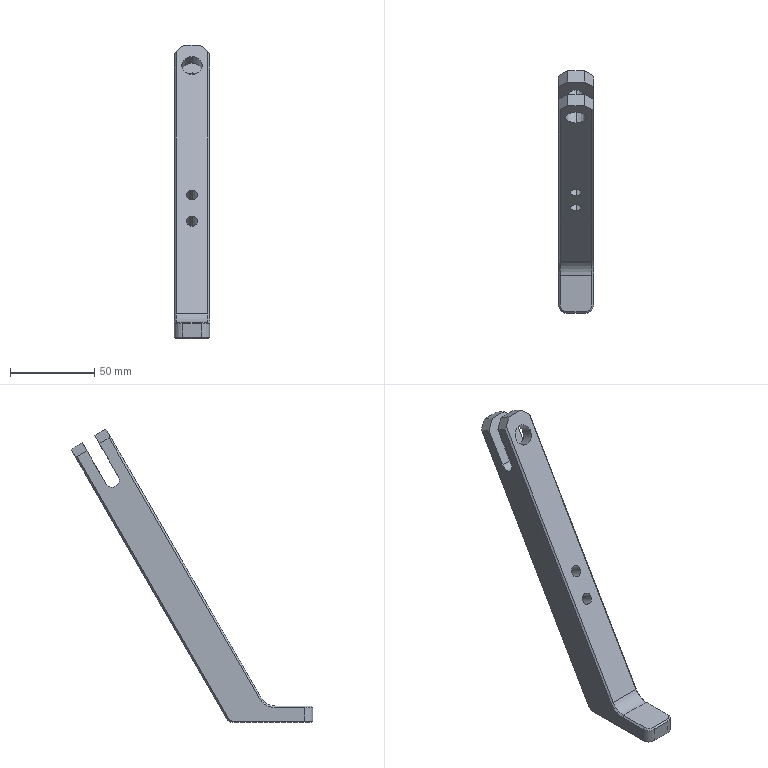Part | SolidWorks | features BaseBody 1 | 1 solid | 86 faces | box 21 x 144 x 174.813 mm | volume 93626 mm3 | cylinder 41 | plane 37 | cone 8 | commonest cylinder face diameters 1.5 x28 6.8 x4 10 x3 8.5 x2 12.2 x2 8.55 x1